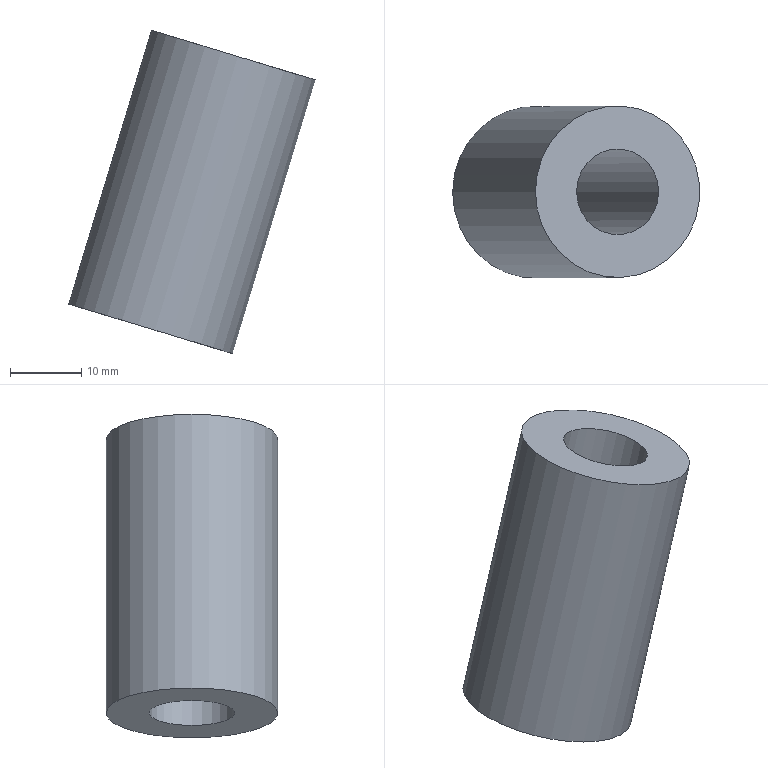Part | STEP file | solid 234 | 1 solid | 4 faces | box 34.555 x 24 x 45.236 mm | volume 13572 mm3 | plane 2 | cylinder 2 | commonest cylinder face diameters 12 x1 24 x1